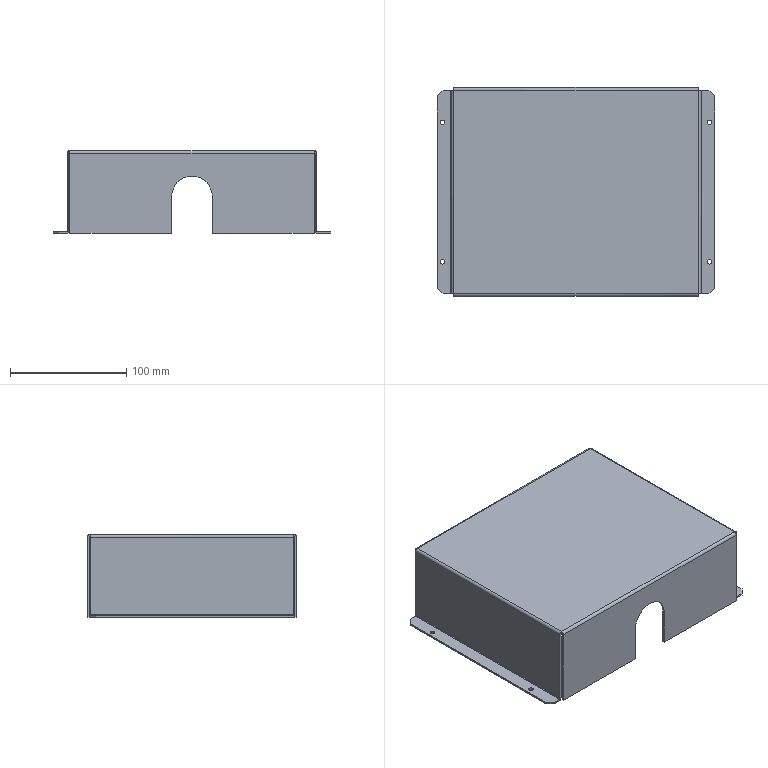Part | NX | 1 solid | 70 faces | box 239 x 180 x 71.5 mm | volume 139409 mm3 | plane 44 | cylinder 18 | spline 8 | commonest cylinder face diameters 1.473 x6 4.473 x6 4 x4 35 x2